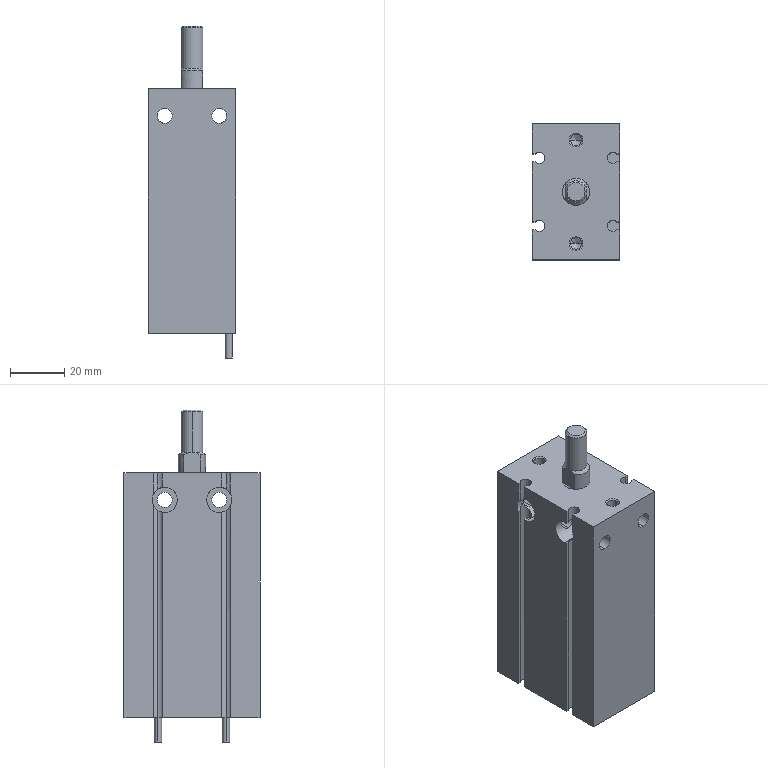Part | STEP file | Bag feed cylinder CDU25-40D-A93L (0) | 1 solid | 139 faces | box 32 x 50 x 122 mm | volume 135464 mm3 | cylinder 60 | plane 51 | cone 28 | commonest cylinder face diameters 5.5 x16 4.134 x12 4.2 x12 9.3 x8 2.7 x4 4 x4